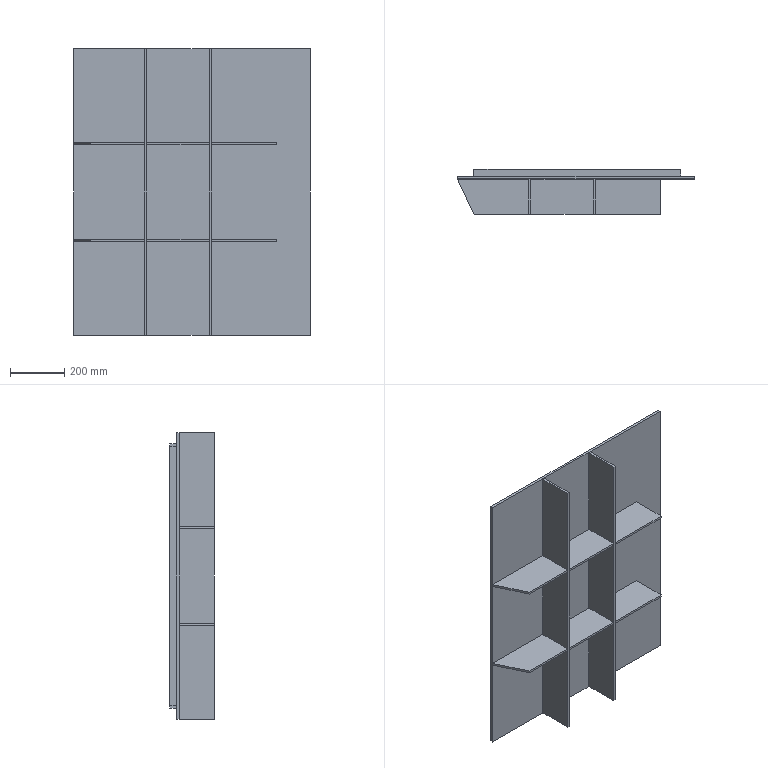Part | STEP file | Grid blind plate_Default<As machined> | 71 solids | 458 faces | box 874.382 x 165 x 1059 mm | volume 15878057 mm3 | plane 458